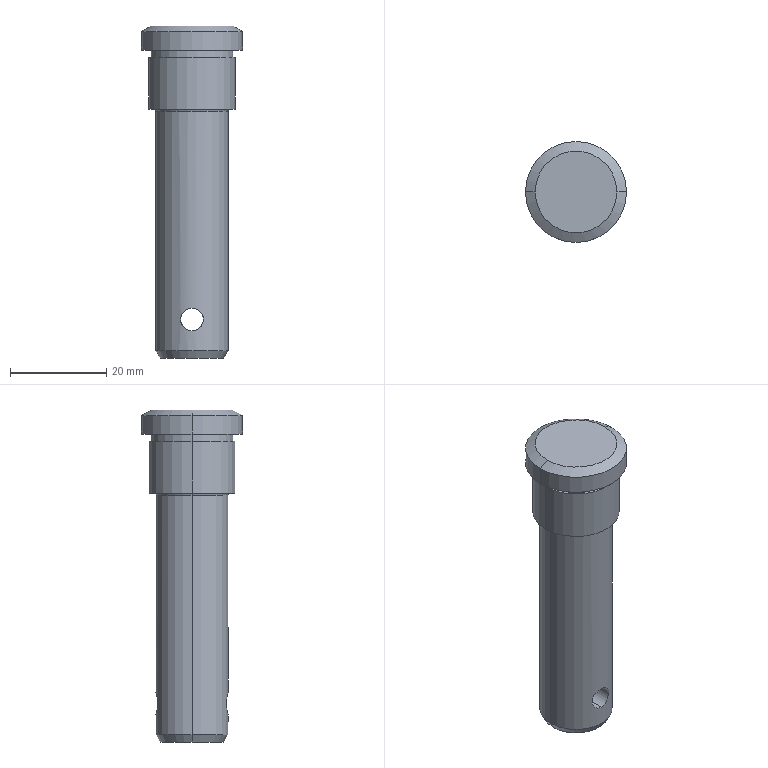Part | STEP file | PERNO POLEA_PERNO V2 | 1 solid | 21 faces | box 21 x 21 x 69 mm | volume 13594 mm3 | cylinder 10 | plane 5 | cone 4 | torus 2 | commonest cylinder face diameters 4.76 x2 15 x2 17 x2 18 x2 21 x2
STEP:
#1=CARTESIAN_POINT('',(7.5,0.,-17.7));
#2=VERTEX_POINT('',#1);
#3=CARTESIAN_POINT('',(-7.5,0.,-17.7));
#4=VERTEX_POINT('',#3);
#5=CARTESIAN_POINT('',(0.,0.,-17.7));
#6=DIRECTION('',(0.,0.,-1.));
#7=DIRECTION('',(-1.,0.,0.));
#8=AXIS2_PLACEMENT_3D('',#5,#6,#7);
#9=CIRCLE('',#8,7.5);
#10=EDGE_CURVE('',#2,#4,#9,.T.);
#11=ORIENTED_EDGE('',*,*,#10,.F.);
#12=CARTESIAN_POINT('',(7.9,0.,-17.3));
#13=VERTEX_POINT('',#12);
#14=CARTESIAN_POINT('',(7.9,0.,-17.7));
#15=DIRECTION('',(0.,1.,0.));
#16=DIRECTION('',(-1.,0.,0.));
#17=AXIS2_PLACEMENT_3D('',#14,#15,#16);
#18=CIRCLE('',#17,0.4);
#19=EDGE_CURVE('',#2,#13,#18,.T.);
#20=ORIENTED_EDGE('',*,*,#19,.T.);
#21=CARTESIAN_POINT('',(-7.9,0.,-17.3));
#22=VERTEX_POINT('',#21);
#23=CARTESIAN_POINT('',(0.,0.,-17.3));
#24=DIRECTION('',(0.,0.,1.));
#25=DIRECTION('',(-1.,0.,0.));
#26=AXIS2_PLACEMENT_3D('',#23,#24,#25);
#27=CIRCLE('',#26,7.9);
#28=EDGE_CURVE('',#22,#13,#27,.T.);
#29=ORIENTED_EDGE('',*,*,#28,.F.);
#30=CARTESIAN_POINT('',(-7.9,0.,-17.7));
#31=DIRECTION('',(0.,-1.,0.));
#32=DIRECTION('',(0.,0.,-1.));
#33=AXIS2_PLACEMENT_3D('',#30,#31,#32);
#34=CIRCLE('',#33,0.4);
#35=EDGE_CURVE('',#4,#22,#34,.T.);
#36=ORIENTED_EDGE('',*,*,#35,.F.);
#37=EDGE_LOOP('',(#11,#20,#29,#36));
#38=FACE_OUTER_BOUND('',#37,.T.);
#39=CARTESIAN_POINT('',(0.,0.,-17.7));
#40=DIRECTION('',(0.,0.,-1.));
#41=DIRECTION('',(-1.,0.,0.));
#42=AXIS2_PLACEMENT_3D('',#39,#40,#41);
#43=TOROIDAL_SURFACE('',#42,7.9,0.4);
#44=ADVANCED_FACE('',(#38),#43,.F.);
#45=CARTESIAN_POINT('',(0.,-7.5,-63.38));
#46=VERTEX_POINT('',#45);
#47=CARTESIAN_POINT('',(0.,-7.5,-58.62));
#48=VERTEX_POINT('',#47);
#49=CARTESIAN_POINT('',(0.,-7.5,-63.38));
#50=CARTESIAN_POINT('',(-0.3119,-7.5,-63.38));
#51=CARTESIAN_POINT('',(-0.6269,-7.479,-63.317));
#52=CARTESIAN_POINT('',(-1.057,-7.426,-63.138));
#53=CARTESIAN_POINT('',(-1.197,-7.405,-63.063));
#54=CARTESIAN_POINT('',(-1.454,-7.359,-62.891));
#55=CARTESIAN_POINT('',(-1.573,-7.334,-62.793));
#56=CARTESIAN_POINT('',(-1.903,-7.258,-62.463));
#57=CARTESIAN_POINT('',(-2.077,-7.208,-62.204));
#58=CARTESIAN_POINT('',(-2.258,-7.152,-61.769));
#59=CARTESIAN_POINT('',(-2.303,-7.138,-61.621));
#60=CARTESIAN_POINT('',(-2.364,-7.118,-61.315));
#61=CARTESIAN_POINT('',(-2.38,-7.112,-61.157));
#62=CARTESIAN_POINT('',(-2.38,-7.112,-60.843));
#63=CARTESIAN_POINT('',(-2.365,-7.118,-60.688));
#64=CARTESIAN_POINT('',(-2.303,-7.138,-60.381));
#65=CARTESIAN_POINT('',(-2.257,-7.153,-60.229));
#66=CARTESIAN_POINT('',(-2.078,-7.207,-59.799));
#67=CARTESIAN_POINT('',(-1.901,-7.258,-59.536));
#68=CARTESIAN_POINT('',(-1.574,-7.334,-59.208));
#69=CARTESIAN_POINT('',(-1.453,-7.359,-59.109));
#70=CARTESIAN_POINT('',(-1.195,-7.405,-58.936));
#71=CARTESIAN_POINT('',(-1.059,-7.426,-58.863));
#72=CARTESIAN_POINT('',(-0.7718,-7.462,-58.743));
#73=CARTESIAN_POINT('',(-0.6199,-7.476,-58.697));
#74=CARTESIAN_POINT('',(-0.314,-7.495,-58.636));
#75=CARTESIAN_POINT('',(-0.1583,-7.5,-58.62));
#76=CARTESIAN_POINT('',(0.,-7.5,-58.62));
#77=B_SPLINE_CURVE_WITH_KNOTS('',3,(#49,#50,#51,#52,#53,#54,#55,#56,#57,#58,#59,#60,#61,#62,#63,#64,#65,#66,#67,#68,#69,#70,#71,#72,#73,#74,#75,#76),.UNSPECIFIED.,.F.,.F.,(4,2,2,2,2,2,2,2,2,2,2,2,2,4),(0.00749,0.008426,0.008894,0.009362,0.0103,0.01077,0.01123,0.0117,0.01217,0.01311,0.01357,0.01404,0.01451,0.01498),.UNSPECIFIED.);
#78=EDGE_CURVE('',#46,#48,#77,.T.);
#79=ORIENTED_EDGE('',*,*,#78,.F.);
#80=CARTESIAN_POINT('',(0.,7.5,-63.38));
#81=VERTEX_POINT('',#80);
#82=CARTESIAN_POINT('',(0.,-10.5,-63.38));
#83=DIRECTION('',(0.,1.,0.));
#84=VECTOR('',#83,1000.);
#85=LINE('',#82,#84);
#86=EDGE_CURVE('',#46,#81,#85,.T.);
#87=ORIENTED_EDGE('',*,*,#86,.T.);
#88=CARTESIAN_POINT('',(0.,7.5,-58.62));
#89=VERTEX_POINT('',#88);
#90=CARTESIAN_POINT('',(0.,7.5,-58.62));
#91=CARTESIAN_POINT('',(-0.1584,7.5,-58.62));
#92=CARTESIAN_POINT('',(-0.3139,7.495,-58.636));
#93=CARTESIAN_POINT('',(-0.6195,7.476,-58.697));
#94=CARTESIAN_POINT('',(-0.7712,7.462,-58.743));
#95=CARTESIAN_POINT('',(-1.059,7.426,-58.863));
#96=CARTESIAN_POINT('',(-1.195,7.405,-58.936));
#97=CARTESIAN_POINT('',(-1.453,7.359,-59.109));
#98=CARTESIAN_POINT('',(-1.575,7.334,-59.209));
#99=CARTESIAN_POINT('',(-1.902,7.258,-59.536));
#100=CARTESIAN_POINT('',(-2.078,7.207,-59.8));
#101=CARTESIAN_POINT('',(-2.257,7.153,-60.229));
#102=CARTESIAN_POINT('',(-2.303,7.138,-60.38));
#103=CARTESIAN_POINT('',(-2.365,7.118,-60.687));
#104=CARTESIAN_POINT('',(-2.38,7.112,-60.842));
#105=CARTESIAN_POINT('',(-2.38,7.112,-61.155));
#106=CARTESIAN_POINT('',(-2.364,7.118,-61.314));
#107=CARTESIAN_POINT('',(-2.303,7.138,-61.62));
#108=CARTESIAN_POINT('',(-2.258,7.152,-61.769));
#109=CARTESIAN_POINT('',(-2.137,7.189,-62.059));
#110=CARTESIAN_POINT('',(-2.063,7.211,-62.196));
#111=CARTESIAN_POINT('',(-1.891,7.258,-62.453));
#112=CARTESIAN_POINT('',(-1.792,7.284,-62.574));
#113=CARTESIAN_POINT('',(-1.573,7.334,-62.793));
#114=CARTESIAN_POINT('',(-1.453,7.359,-62.891));
#115=CARTESIAN_POINT('',(-1.196,7.405,-63.063));
#116=CARTESIAN_POINT('',(-1.057,7.427,-63.138));
#117=CARTESIAN_POINT('',(-0.7702,7.462,-63.257));
#118=CARTESIAN_POINT('',(-0.6217,7.476,-63.303));
#119=CARTESIAN_POINT('',(-0.3139,7.495,-63.364));
#120=CARTESIAN_POINT('',(-0.156,7.5,-63.38));
#121=CARTESIAN_POINT('',(0.,7.5,-63.38));
#122=B_SPLINE_CURVE_WITH_KNOTS('',3,(#90,#91,#92,#93,#94,#95,#96,#97,#98,#99,#100,#101,#102,#103,#104,#105,#106,#107,#108,#109,#110,#111,#112,#113,#114,#115,#116,#117,#118,#119,#120,#121),.UNSPECIFIED.,.F.,.F.,(4,2,2,2,2,2,2,2,2,2,2,2,2,2,2,4),(0.,0.0004681,0.0009362,0.001404,0.001872,0.002809,0.003277,0.003745,0.004213,0.004681,0.005149,0.005617,0.006085,0.006553,0.007022,0.00749),.UNSPECIFIED.);
#123=EDGE_CURVE('',#89,#81,#122,.T.);
#124=ORIENTED_EDGE('',*,*,#123,.F.);
#125=CARTESIAN_POINT('',(0.,-10.5,-58.62));
#126=DIRECTION('',(0.,1.,0.));
#127=VECTOR('',#126,1000.);
#128=LINE('',#125,#127);
#129=EDGE_CURVE('',#48,#89,#128,.T.);
#130=ORIENTED_EDGE('',*,*,#129,.F.);
#131=EDGE_LOOP('',(#79,#87,#124,#130));
#132=FACE_OUTER_BOUND('',#131,.T.);
#133=CARTESIAN_POINT('',(0.,-10.5,-61.));
#134=DIRECTION('',(0.,1.,0.));
#135=DIRECTION('',(0.,0.,1.));
#136=AXIS2_PLACEMENT_3D('',#133,#134,#135);
#137=CYLINDRICAL_SURFACE('',#136,2.38);
#138=ADVANCED_FACE('',(#132),#137,.F.);
#139=CARTESIAN_POINT('',(-6.634,0.,-69.));
#140=VERTEX_POINT('',#139);
#141=CARTESIAN_POINT('',(6.634,0.,-69.));
#142=VERTEX_POINT('',#141);
#143=CARTESIAN_POINT('',(0.,0.,-69.));
#144=DIRECTION('',(0.,0.,-1.));
#145=DIRECTION('',(1.,0.,0.));
#146=AXIS2_PLACEMENT_3D('',#143,#144,#145);
#147=CIRCLE('',#146,6.634);
#148=EDGE_CURVE('',#140,#142,#147,.T.);
#149=ORIENTED_EDGE('',*,*,#148,.F.);
#150=CARTESIAN_POINT('',(-7.5,0.,-67.5));
#151=VERTEX_POINT('',#150);
#152=CARTESIAN_POINT('',(-7.5,0.,-67.5));
#153=DIRECTION('',(-0.5,0.,0.866));
#154=VECTOR('',#153,1000.);
#155=LINE('',#152,#154);
#156=EDGE_CURVE('',#140,#151,#155,.T.);
#157=ORIENTED_EDGE('',*,*,#156,.T.);
#158=CARTESIAN_POINT('',(7.5,0.,-67.5));
#159=VERTEX_POINT('',#158);
#160=CARTESIAN_POINT('',(0.,0.,-67.5));
#161=DIRECTION('',(0.,0.,1.));
#162=DIRECTION('',(1.,0.,0.));
#163=AXIS2_PLACEMENT_3D('',#160,#161,#162);
#164=CIRCLE('',#163,7.5);
#165=EDGE_CURVE('',#159,#151,#164,.T.);
#166=ORIENTED_EDGE('',*,*,#165,.F.);
#167=CARTESIAN_POINT('',(7.5,0.,-67.5));
#168=DIRECTION('',(0.5,0.,0.866));
#169=VECTOR('',#168,1000.);
#170=LINE('',#167,#169);
#171=EDGE_CURVE('',#142,#159,#170,.T.);
#172=ORIENTED_EDGE('',*,*,#171,.F.);
#173=EDGE_LOOP('',(#149,#157,#166,#172));
#174=FACE_OUTER_BOUND('',#173,.T.);
#175=CARTESIAN_POINT('',(0.,0.,-67.5));
#176=DIRECTION('',(0.,0.,1.));
#177=DIRECTION('',(1.,0.,0.));
#178=AXIS2_PLACEMENT_3D('',#175,#176,#177);
#179=CONICAL_SURFACE('',#178,7.5,0.5236);
#180=ADVANCED_FACE('',(#174),#179,.T.);
#181=CARTESIAN_POINT('',(8.5,0.,0.));
#182=VERTEX_POINT('',#181);
#183=CARTESIAN_POINT('',(-8.5,0.,0.));
#184=VERTEX_POINT('',#183);
#185=CARTESIAN_POINT('',(0.,0.,0.));
#186=DIRECTION('',(0.,0.,1.));
#187=DIRECTION('',(-1.,0.,0.));
#188=AXIS2_PLACEMENT_3D('',#185,#186,#187);
#189=CIRCLE('',#188,8.5);
#190=EDGE_CURVE('',#182,#184,#189,.T.);
#191=ORIENTED_EDGE('',*,*,#190,.F.);
#192=CARTESIAN_POINT('',(10.5,0.,-1.155));
#193=VERTEX_POINT('',#192);
#194=CARTESIAN_POINT('',(8.5,0.,0.));
#195=DIRECTION('',(0.866,0.,-0.5));
#196=VECTOR('',#195,1000.);
#197=LINE('',#194,#196);
#198=EDGE_CURVE('',#182,#193,#197,.T.);
#199=ORIENTED_EDGE('',*,*,#198,.T.);
#200=CARTESIAN_POINT('',(-10.5,0.,-1.155));
#201=VERTEX_POINT('',#200);
#202=CARTESIAN_POINT('',(0.,0.,-1.155));
#203=DIRECTION('',(0.,0.,-1.));
#204=DIRECTION('',(-1.,0.,0.));
#205=AXIS2_PLACEMENT_3D('',#202,#203,#204);
#206=CIRCLE('',#205,10.5);
#207=EDGE_CURVE('',#201,#193,#206,.T.);
#208=ORIENTED_EDGE('',*,*,#207,.F.);
#209=CARTESIAN_POINT('',(-8.5,0.,0.));
#210=DIRECTION('',(-0.866,0.,-0.5));
#211=VECTOR('',#210,1000.);
#212=LINE('',#209,#211);
#213=EDGE_CURVE('',#184,#201,#212,.T.);
#214=ORIENTED_EDGE('',*,*,#213,.F.);
#215=EDGE_LOOP('',(#191,#199,#208,#214));
#216=FACE_OUTER_BOUND('',#215,.T.);
#217=CARTESIAN_POINT('',(0.,0.,0.));
#218=DIRECTION('',(0.,0.,-1.));
#219=DIRECTION('',(-1.,0.,0.));
#220=AXIS2_PLACEMENT_3D('',#217,#218,#219);
#221=CONICAL_SURFACE('',#220,8.5,1.047);
#222=ADVANCED_FACE('',(#216),#221,.T.);
#223=CARTESIAN_POINT('',(10.5,0.,-5.));
#224=VERTEX_POINT('',#223);
#225=CARTESIAN_POINT('',(-10.5,0.,-5.));
#226=VERTEX_POINT('',#225);
#227=CARTESIAN_POINT('',(0.,0.,-5.));
#228=DIRECTION('',(0.,0.,1.));
#229=DIRECTION('',(1.,0.,0.));
#230=AXIS2_PLACEMENT_3D('',#227,#228,#229);
#231=CIRCLE('',#230,10.5);
#232=EDGE_CURVE('',#224,#226,#231,.T.);
#233=ORIENTED_EDGE('',*,*,#232,.T.);
#234=CARTESIAN_POINT('',(-10.5,0.,0.));
#235=DIRECTION('',(0.,0.,1.));
#236=VECTOR('',#235,1000.);
#237=LINE('',#234,#236);
#238=EDGE_CURVE('',#226,#201,#237,.T.);
#239=ORIENTED_EDGE('',*,*,#238,.T.);
#240=ORIENTED_EDGE('',*,*,#207,.T.);
#241=CARTESIAN_POINT('',(10.5,0.,0.));
#242=DIRECTION('',(0.,0.,1.));
#243=VECTOR('',#242,1000.);
#244=LINE('',#241,#243);
#245=EDGE_CURVE('',#224,#193,#244,.T.);
#246=ORIENTED_EDGE('',*,*,#245,.F.);
#247=EDGE_LOOP('',(#233,#239,#240,#246));
#248=FACE_OUTER_BOUND('',#247,.T.);
#249=CARTESIAN_POINT('',(0.,0.,0.));
#250=DIRECTION('',(0.,0.,1.));
#251=DIRECTION('',(1.,0.,0.));
#252=AXIS2_PLACEMENT_3D('',#249,#250,#251);
#253=CYLINDRICAL_SURFACE('',#252,10.5);
#254=ADVANCED_FACE('',(#248),#253,.T.);
#255=CARTESIAN_POINT('',(8.5,0.,-6.5));
#256=VERTEX_POINT('',#255);
#257=CARTESIAN_POINT('',(-8.5,0.,-6.5));
#258=VERTEX_POINT('',#257);
#259=CARTESIAN_POINT('',(0.,0.,-6.5));
#260=DIRECTION('',(0.,0.,1.));
#261=DIRECTION('',(1.,0.,0.));
#262=AXIS2_PLACEMENT_3D('',#259,#260,#261);
#263=CIRCLE('',#262,8.5);
#264=EDGE_CURVE('',#256,#258,#263,.T.);
#265=ORIENTED_EDGE('',*,*,#264,.T.);
#266=CARTESIAN_POINT('',(-8.5,0.,-5.));
#267=VERTEX_POINT('',#266);
#268=CARTESIAN_POINT('',(-8.5,0.,0.));
#269=DIRECTION('',(0.,0.,1.));
#270=VECTOR('',#269,1000.);
#271=LINE('',#268,#270);
#272=EDGE_CURVE('',#258,#267,#271,.T.);
#273=ORIENTED_EDGE('',*,*,#272,.T.);
#274=CARTESIAN_POINT('',(8.5,0.,-5.));
#275=VERTEX_POINT('',#274);
#276=CARTESIAN_POINT('',(0.,0.,-5.));
#277=DIRECTION('',(0.,0.,1.));
#278=DIRECTION('',(1.,0.,0.));
#279=AXIS2_PLACEMENT_3D('',#276,#277,#278);
#280=CIRCLE('',#279,8.5);
#281=EDGE_CURVE('',#275,#267,#280,.T.);
#282=ORIENTED_EDGE('',*,*,#281,.F.);
#283=CARTESIAN_POINT('',(8.5,0.,0.));
#284=DIRECTION('',(0.,0.,1.));
#285=VECTOR('',#284,1000.);
#286=LINE('',#283,#285);
#287=EDGE_CURVE('',#256,#275,#286,.T.);
#288=ORIENTED_EDGE('',*,*,#287,.F.);
#289=EDGE_LOOP('',(#265,#273,#282,#288));
#290=FACE_OUTER_BOUND('',#289,.T.);
#291=CARTESIAN_POINT('',(0.,0.,0.));
#292=DIRECTION('',(0.,0.,1.));
#293=DIRECTION('',(1.,0.,0.));
#294=AXIS2_PLACEMENT_3D('',#291,#292,#293);
#295=CYLINDRICAL_SURFACE('',#294,8.5);
#296=ADVANCED_FACE('',(#290),#295,.T.);
#297=ORIENTED_EDGE('',*,*,#123,.T.);
#298=CARTESIAN_POINT('',(0.,7.5,-63.38));
#299=CARTESIAN_POINT('',(0.3119,7.5,-63.38));
#300=CARTESIAN_POINT('',(0.6269,7.479,-63.317));
#301=CARTESIAN_POINT('',(1.057,7.426,-63.138));
#302=CARTESIAN_POINT('',(1.197,7.405,-63.063));
#303=CARTESIAN_POINT('',(1.454,7.359,-62.891));
#304=CARTESIAN_POINT('',(1.573,7.334,-62.793));
#305=CARTESIAN_POINT('',(1.903,7.258,-62.463));
#306=CARTESIAN_POINT('',(2.077,7.208,-62.204));
#307=CARTESIAN_POINT('',(2.258,7.152,-61.769));
#308=CARTESIAN_POINT('',(2.303,7.138,-61.621));
#309=CARTESIAN_POINT('',(2.364,7.118,-61.315));
#310=CARTESIAN_POINT('',(2.38,7.112,-61.157));
#311=CARTESIAN_POINT('',(2.38,7.112,-60.843));
#312=CARTESIAN_POINT('',(2.365,7.118,-60.688));
#313=CARTESIAN_POINT('',(2.303,7.138,-60.381));
#314=CARTESIAN_POINT('',(2.257,7.153,-60.229));
#315=CARTESIAN_POINT('',(2.078,7.207,-59.799));
#316=CARTESIAN_POINT('',(1.901,7.258,-59.536));
#317=CARTESIAN_POINT('',(1.574,7.334,-59.208));
#318=CARTESIAN_POINT('',(1.453,7.359,-59.109));
#319=CARTESIAN_POINT('',(1.195,7.405,-58.936));
#320=CARTESIAN_POINT('',(1.059,7.426,-58.863));
#321=CARTESIAN_POINT('',(0.7718,7.462,-58.743));
#322=CARTESIAN_POINT('',(0.6199,7.476,-58.697));
#323=CARTESIAN_POINT('',(0.314,7.495,-58.636));
#324=CARTESIAN_POINT('',(0.1583,7.5,-58.62));
#325=CARTESIAN_POINT('',(0.,7.5,-58.62));
#326=B_SPLINE_CURVE_WITH_KNOTS('',3,(#298,#299,#300,#301,#302,#303,#304,#305,#306,#307,#308,#309,#310,#311,#312,#313,#314,#315,#316,#317,#318,#319,#320,#321,#322,#323,#324,#325),.UNSPECIFIED.,.F.,.F.,(4,2,2,2,2,2,2,2,2,2,2,2,2,4),(0.00749,0.008426,0.008894,0.009362,0.0103,0.01077,0.01123,0.0117,0.01217,0.01311,0.01357,0.01404,0.01451,0.01498),.UNSPECIFIED.);
#327=EDGE_CURVE('',#81,#89,#326,.T.);
#328=ORIENTED_EDGE('',*,*,#327,.T.);
#329=EDGE_LOOP('',(#297,#328));
#330=FACE_BOUND('',#329,.T.);
#331=ORIENTED_EDGE('',*,*,#165,.T.);
#332=CARTESIAN_POINT('',(-7.5,0.,0.));
#333=DIRECTION('',(0.,0.,1.));
#334=VECTOR('',#333,1000.);
#335=LINE('',#332,#334);
#336=EDGE_CURVE('',#151,#4,#335,.T.);
#337=ORIENTED_EDGE('',*,*,#336,.T.);
#338=CARTESIAN_POINT('',(0.,0.,-17.7));
#339=DIRECTION('',(0.,0.,-1.));
#340=DIRECTION('',(-1.,0.,0.));
#341=AXIS2_PLACEMENT_3D('',#338,#339,#340);
#342=CIRCLE('',#341,7.5);
#343=EDGE_CURVE('',#4,#2,#342,.T.);
#344=ORIENTED_EDGE('',*,*,#343,.T.);
#345=CARTESIAN_POINT('',(7.5,0.,0.));
#346=DIRECTION('',(0.,0.,1.));
#347=VECTOR('',#346,1000.);
#348=LINE('',#345,#347);
#349=EDGE_CURVE('',#159,#2,#348,.T.);
#350=ORIENTED_EDGE('',*,*,#349,.F.);
#351=EDGE_LOOP('',(#331,#337,#344,#350));
#352=FACE_OUTER_BOUND('',#351,.T.);
#353=CARTESIAN_POINT('',(0.,0.,0.));
#354=DIRECTION('',(0.,0.,1.));
#355=DIRECTION('',(1.,0.,0.));
#356=AXIS2_PLACEMENT_3D('',#353,#354,#355);
#357=CYLINDRICAL_SURFACE('',#356,7.5);
#358=ADVANCED_FACE('',(#330,#352),#357,.T.);
#359=CARTESIAN_POINT('',(-9.,0.,-17.3));
#360=VERTEX_POINT('',#359);
#361=CARTESIAN_POINT('',(9.,0.,-17.3));
#362=VERTEX_POINT('',#361);
#363=CARTESIAN_POINT('',(0.,0.,-17.3));
#364=DIRECTION('',(0.,0.,-1.));
#365=DIRECTION('',(-1.,0.,0.));
#366=AXIS2_PLACEMENT_3D('',#363,#364,#365);
#367=CIRCLE('',#366,9.);
#368=EDGE_CURVE('',#360,#362,#367,.T.);
#369=ORIENTED_EDGE('',*,*,#368,.F.);
#370=CARTESIAN_POINT('',(-9.,0.,-6.5));
#371=VERTEX_POINT('',#370);
#372=CARTESIAN_POINT('',(-9.,0.,-17.3));
#373=DIRECTION('',(0.,0.,1.));
#374=VECTOR('',#373,1000.);
#375=LINE('',#372,#374);
#376=EDGE_CURVE('',#360,#371,#375,.T.);
#377=ORIENTED_EDGE('',*,*,#376,.T.);
#378=CARTESIAN_POINT('',(9.,0.,-6.5));
#379=VERTEX_POINT('',#378);
#380=CARTESIAN_POINT('',(0.,0.,-6.5));
#381=DIRECTION('',(0.,0.,1.));
#382=DIRECTION('',(1.,0.,0.));
#383=AXIS2_PLACEMENT_3D('',#380,#381,#382);
#384=CIRCLE('',#383,9.);
#385=EDGE_CURVE('',#379,#371,#384,.T.);
#386=ORIENTED_EDGE('',*,*,#385,.F.);
#387=CARTESIAN_POINT('',(9.,0.,-17.3));
#388=DIRECTION('',(0.,0.,1.));
#389=VECTOR('',#388,1000.);
#390=LINE('',#387,#389);
#391=EDGE_CURVE('',#362,#379,#390,.T.);
#392=ORIENTED_EDGE('',*,*,#391,.F.);
#393=EDGE_LOOP('',(#369,#377,#386,#392));
#394=FACE_OUTER_BOUND('',#393,.T.);
#395=CARTESIAN_POINT('',(0.,0.,-17.3));
#396=DIRECTION('',(0.,0.,1.));
#397=DIRECTION('',(1.,0.,0.));
#398=AXIS2_PLACEMENT_3D('',#395,#396,#397);
#399=CYLINDRICAL_SURFACE('',#398,9.);
#400=ADVANCED_FACE('',(#394),#399,.T.);
#401=ORIENTED_EDGE('',*,*,#376,.F.);
#402=CARTESIAN_POINT('',(0.,0.,-17.3));
#403=DIRECTION('',(0.,0.,-1.));
#404=DIRECTION('',(-1.,0.,0.));
#405=AXIS2_PLACEMENT_3D('',#402,#403,#404);
#406=CIRCLE('',#405,9.);
#407=EDGE_CURVE('',#362,#360,#406,.T.);
#408=ORIENTED_EDGE('',*,*,#407,.F.);
#409=ORIENTED_EDGE('',*,*,#391,.T.);
#410=CARTESIAN_POINT('',(0.,0.,-6.5));
#411=DIRECTION('',(0.,0.,1.));
#412=DIRECTION('',(1.,0.,0.));
#413=AXIS2_PLACEMENT_3D('',#410,#411,#412);
#414=CIRCLE('',#413,9.);
#415=EDGE_CURVE('',#371,#379,#414,.T.);
#416=ORIENTED_EDGE('',*,*,#415,.F.);
#417=EDGE_LOOP('',(#401,#408,#409,#416));
#418=FACE_OUTER_BOUND('',#417,.T.);
#419=CARTESIAN_POINT('',(0.,0.,-17.3));
#420=DIRECTION('',(0.,0.,1.));
#421=DIRECTION('',(1.,0.,0.));
#422=AXIS2_PLACEMENT_3D('',#419,#420,#421);
#423=CYLINDRICAL_SURFACE('',#422,9.);
#424=ADVANCED_FACE('',(#418),#423,.T.);
#425=ORIENTED_EDGE('',*,*,#28,.T.);
#426=CARTESIAN_POINT('',(0.,0.,-17.3));
#427=DIRECTION('',(0.,0.,1.));
#428=DIRECTION('',(-1.,0.,0.));
#429=AXIS2_PLACEMENT_3D('',#426,#427,#428);
#430=CIRCLE('',#429,7.9);
#431=EDGE_CURVE('',#13,#22,#430,.T.);
#432=ORIENTED_EDGE('',*,*,#431,.T.);
#433=EDGE_LOOP('',(#425,#432));
#434=FACE_BOUND('',#433,.T.);
#435=ORIENTED_EDGE('',*,*,#407,.T.);
#436=ORIENTED_EDGE('',*,*,#368,.T.);
#437=EDGE_LOOP('',(#435,#436));
#438=FACE_OUTER_BOUND('',#437,.T.);
#439=CARTESIAN_POINT('',(0.,0.,-17.3));
#440=DIRECTION('',(0.,0.,-1.));
#441=DIRECTION('',(-1.,0.,0.));
#442=AXIS2_PLACEMENT_3D('',#439,#440,#441);
#443=PLANE('',#442);
#444=ADVANCED_FACE('',(#434,#438),#443,.T.);
#445=CARTESIAN_POINT('',(0.,0.,-69.));
#446=DIRECTION('',(0.,0.,-1.));
#447=DIRECTION('',(1.,0.,0.));
#448=AXIS2_PLACEMENT_3D('',#445,#446,#447);
#449=CIRCLE('',#448,6.634);
#450=EDGE_CURVE('',#142,#140,#449,.T.);
#451=ORIENTED_EDGE('',*,*,#450,.T.);
#452=ORIENTED_EDGE('',*,*,#148,.T.);
#453=EDGE_LOOP('',(#451,#452));
#454=FACE_OUTER_BOUND('',#453,.T.);
#455=CARTESIAN_POINT('',(0.,7.5,-69.));
#456=DIRECTION('',(0.,0.,1.));
#457=DIRECTION('',(1.,0.,0.));
#458=AXIS2_PLACEMENT_3D('',#455,#456,#457);
#459=PLANE('',#458);
#460=ADVANCED_FACE('',(#454),#459,.F.);
#461=ORIENTED_EDGE('',*,*,#336,.F.);
#462=CARTESIAN_POINT('',(0.,0.,-67.5));
#463=DIRECTION('',(0.,0.,1.));
#464=DIRECTION('',(1.,0.,0.));
#465=AXIS2_PLACEMENT_3D('',#462,#463,#464);
#466=CIRCLE('',#465,7.5);
#467=EDGE_CURVE('',#151,#159,#466,.T.);
#468=ORIENTED_EDGE('',*,*,#467,.T.);
#469=ORIENTED_EDGE('',*,*,#349,.T.);
#470=ORIENTED_EDGE('',*,*,#10,.T.);
#471=EDGE_LOOP('',(#461,#468,#469,#470));
#472=FACE_OUTER_BOUND('',#471,.T.);
#473=CARTESIAN_POINT('',(0.,-7.5,-58.62));
#474=CARTESIAN_POINT('',(0.1584,-7.5,-58.62));
#475=CARTESIAN_POINT('',(0.3139,-7.495,-58.636));
#476=CARTESIAN_POINT('',(0.6195,-7.476,-58.697));
#477=CARTESIAN_POINT('',(0.7712,-7.462,-58.743));
#478=CARTESIAN_POINT('',(1.059,-7.426,-58.863));
#479=CARTESIAN_POINT('',(1.195,-7.405,-58.936));
#480=CARTESIAN_POINT('',(1.453,-7.359,-59.109));
#481=CARTESIAN_POINT('',(1.575,-7.334,-59.209));
#482=CARTESIAN_POINT('',(1.902,-7.258,-59.536));
#483=CARTESIAN_POINT('',(2.078,-7.207,-59.8));
#484=CARTESIAN_POINT('',(2.257,-7.153,-60.229));
#485=CARTESIAN_POINT('',(2.303,-7.138,-60.38));
#486=CARTESIAN_POINT('',(2.365,-7.118,-60.687));
#487=CARTESIAN_POINT('',(2.38,-7.112,-60.842));
#488=CARTESIAN_POINT('',(2.38,-7.112,-61.155));
#489=CARTESIAN_POINT('',(2.364,-7.118,-61.314));
#490=CARTESIAN_POINT('',(2.303,-7.138,-61.62));
#491=CARTESIAN_POINT('',(2.258,-7.152,-61.769));
#492=CARTESIAN_POINT('',(2.137,-7.189,-62.059));
#493=CARTESIAN_POINT('',(2.063,-7.211,-62.196));
#494=CARTESIAN_POINT('',(1.891,-7.258,-62.453));
#495=CARTESIAN_POINT('',(1.792,-7.284,-62.574));
#496=CARTESIAN_POINT('',(1.573,-7.334,-62.793));
#497=CARTESIAN_POINT('',(1.453,-7.359,-62.891));
#498=CARTESIAN_POINT('',(1.196,-7.405,-63.063));
#499=CARTESIAN_POINT('',(1.057,-7.427,-63.138));
#500=CARTESIAN_POINT('',(0.7702,-7.462,-63.257));
#501=CARTESIAN_POINT('',(0.6217,-7.476,-63.303));
#502=CARTESIAN_POINT('',(0.3139,-7.495,-63.364));
#503=CARTESIAN_POINT('',(0.156,-7.5,-63.38));
#504=CARTESIAN_POINT('',(0.,-7.5,-63.38));
#505=B_SPLINE_CURVE_WITH_KNOTS('',3,(#473,#474,#475,#476,#477,#478,#479,#480,#481,#482,#483,#484,#485,#486,#487,#488,#489,#490,#491,#492,#493,#494,#495,#496,#497,#498,#499,#500,#501,#502,#503,#504),.UNSPECIFIED.,.F.,.F.,(4,2,2,2,2,2,2,2,2,2,2,2,2,2,2,4),(0.,0.0004681,0.0009362,0.001404,0.001872,0.002809,0.003277,0.003745,0.004213,0.004681,0.005149,0.005617,0.006085,0.006553,0.007022,0.00749),.UNSPECIFIED.);
#506=EDGE_CURVE('',#48,#46,#505,.T.);
#507=ORIENTED_EDGE('',*,*,#506,.T.);
#508=ORIENTED_EDGE('',*,*,#78,.T.);
#509=EDGE_LOOP('',(#507,#508));
#510=FACE_BOUND('',#509,.T.);
#511=CARTESIAN_POINT('',(0.,0.,0.));
#512=DIRECTION('',(0.,0.,1.));
#513=DIRECTION('',(1.,0.,0.));
#514=AXIS2_PLACEMENT_3D('',#511,#512,#513);
#515=CYLINDRICAL_SURFACE('',#514,7.5);
#516=ADVANCED_FACE('',(#472,#510),#515,.T.);
#517=ORIENTED_EDGE('',*,*,#264,.F.);
#518=CARTESIAN_POINT('',(0.,0.,-6.5));
#519=DIRECTION('',(0.,0.,1.));
#520=DIRECTION('',(1.,0.,0.));
#521=AXIS2_PLACEMENT_3D('',#518,#519,#520);
#522=CIRCLE('',#521,8.5);
#523=EDGE_CURVE('',#258,#256,#522,.T.);
#524=ORIENTED_EDGE('',*,*,#523,.F.);
#525=EDGE_LOOP('',(#517,#524));
#526=FACE_BOUND('',#525,.T.);
#527=ORIENTED_EDGE('',*,*,#385,.T.);
#528=ORIENTED_EDGE('',*,*,#415,.T.);
#529=EDGE_LOOP('',(#527,#528));
#530=FACE_OUTER_BOUND('',#529,.T.);
#531=CARTESIAN_POINT('',(-23.264,0.,-6.5));
#532=DIRECTION('',(0.,0.,1.));
#533=DIRECTION('',(1.,0.,0.));
#534=AXIS2_PLACEMENT_3D('',#531,#532,#533);
#535=PLANE('',#534);
#536=ADVANCED_FACE('',(#526,#530),#535,.T.);
#537=ORIENTED_EDGE('',*,*,#272,.F.);
#538=ORIENTED_EDGE('',*,*,#523,.T.);
#539=ORIENTED_EDGE('',*,*,#287,.T.);
#540=CARTESIAN_POINT('',(0.,0.,-5.));
#541=DIRECTION('',(0.,0.,1.));
#542=DIRECTION('',(1.,0.,0.));
#543=AXIS2_PLACEMENT_3D('',#540,#541,#542);
#544=CIRCLE('',#543,8.5);
#545=EDGE_CURVE('',#267,#275,#544,.T.);
#546=ORIENTED_EDGE('',*,*,#545,.F.);
#547=EDGE_LOOP('',(#537,#538,#539,#546));
#548=FACE_OUTER_BOUND('',#547,.T.);
#549=CARTESIAN_POINT('',(0.,0.,0.));
#550=DIRECTION('',(0.,0.,1.));
#551=DIRECTION('',(1.,0.,0.));
#552=AXIS2_PLACEMENT_3D('',#549,#550,#551);
#553=CYLINDRICAL_SURFACE('',#552,8.5);
#554=ADVANCED_FACE('',(#548),#553,.T.);
#555=CARTESIAN_POINT('',(0.,0.,0.));
#556=DIRECTION('',(0.,0.,1.));
#557=DIRECTION('',(-1.,0.,0.));
#558=AXIS2_PLACEMENT_3D('',#555,#556,#557);
#559=CIRCLE('',#558,8.5);
#560=EDGE_CURVE('',#184,#182,#559,.T.);
#561=ORIENTED_EDGE('',*,*,#560,.T.);
#562=ORIENTED_EDGE('',*,*,#190,.T.);
#563=EDGE_LOOP('',(#561,#562));
#564=FACE_OUTER_BOUND('',#563,.T.);
#565=CARTESIAN_POINT('',(0.,0.,0.));
#566=DIRECTION('',(0.,0.,-1.));
#567=DIRECTION('',(-1.,0.,0.));
#568=AXIS2_PLACEMENT_3D('',#565,#566,#567);
#569=PLANE('',#568);
#570=ADVANCED_FACE('',(#564),#569,.F.);
#571=ORIENTED_EDGE('',*,*,#238,.F.);
#572=CARTESIAN_POINT('',(0.,0.,-5.));
#573=DIRECTION('',(0.,0.,1.));
#574=DIRECTION('',(1.,0.,0.));
#575=AXIS2_PLACEMENT_3D('',#572,#573,#574);
#576=CIRCLE('',#575,10.5);
#577=EDGE_CURVE('',#226,#224,#576,.T.);
#578=ORIENTED_EDGE('',*,*,#577,.T.);
#579=ORIENTED_EDGE('',*,*,#245,.T.);
#580=CARTESIAN_POINT('',(0.,0.,-1.155));
#581=DIRECTION('',(0.,0.,-1.));
#582=DIRECTION('',(-1.,0.,0.));
#583=AXIS2_PLACEMENT_3D('',#580,#581,#582);
#584=CIRCLE('',#583,10.5);
#585=EDGE_CURVE('',#193,#201,#584,.T.);
#586=ORIENTED_EDGE('',*,*,#585,.T.);
#587=EDGE_LOOP('',(#571,#578,#579,#586));
#588=FACE_OUTER_BOUND('',#587,.T.);
#589=CARTESIAN_POINT('',(0.,0.,0.));
#590=DIRECTION('',(0.,0.,1.));
#591=DIRECTION('',(1.,0.,0.));
#592=AXIS2_PLACEMENT_3D('',#589,#590,#591);
#593=CYLINDRICAL_SURFACE('',#592,10.5);
#594=ADVANCED_FACE('',(#588),#593,.T.);
#595=ORIENTED_EDGE('',*,*,#232,.F.);
#596=ORIENTED_EDGE('',*,*,#577,.F.);
#597=EDGE_LOOP('',(#595,#596));
#598=FACE_OUTER_BOUND('',#597,.T.);
#599=ORIENTED_EDGE('',*,*,#281,.T.);
#600=ORIENTED_EDGE('',*,*,#545,.T.);
#601=EDGE_LOOP('',(#599,#600));
#602=FACE_BOUND('',#601,.T.);
#603=CARTESIAN_POINT('',(0.,10.5,-5.));
#604=DIRECTION('',(0.,0.,1.));
#605=DIRECTION('',(1.,0.,0.));
#606=AXIS2_PLACEMENT_3D('',#603,#604,#605);
#607=PLANE('',#606);
#608=ADVANCED_FACE('',(#598,#602),#607,.F.);
#609=ORIENTED_EDGE('',*,*,#198,.F.);
#610=ORIENTED_EDGE('',*,*,#560,.F.);
#611=ORIENTED_EDGE('',*,*,#213,.T.);
#612=ORIENTED_EDGE('',*,*,#585,.F.);
#613=EDGE_LOOP('',(#609,#610,#611,#612));
#614=FACE_OUTER_BOUND('',#613,.T.);
#615=CARTESIAN_POINT('',(0.,0.,0.));
#616=DIRECTION('',(0.,0.,-1.));
#617=DIRECTION('',(-1.,0.,0.));
#618=AXIS2_PLACEMENT_3D('',#615,#616,#617);
#619=CONICAL_SURFACE('',#618,8.5,1.047);
#620=ADVANCED_FACE('',(#614),#619,.T.);
#621=ORIENTED_EDGE('',*,*,#156,.F.);
#622=ORIENTED_EDGE('',*,*,#450,.F.);
#623=ORIENTED_EDGE('',*,*,#171,.T.);
#624=ORIENTED_EDGE('',*,*,#467,.F.);
#625=EDGE_LOOP('',(#621,#622,#623,#624));
#626=FACE_OUTER_BOUND('',#625,.T.);
#627=CARTESIAN_POINT('',(0.,0.,-67.5));
#628=DIRECTION('',(0.,0.,1.));
#629=DIRECTION('',(1.,0.,0.));
#630=AXIS2_PLACEMENT_3D('',#627,#628,#629);
#631=CONICAL_SURFACE('',#630,7.5,0.5236);
#632=ADVANCED_FACE('',(#626),#631,.T.);
#633=ORIENTED_EDGE('',*,*,#86,.F.);
#634=ORIENTED_EDGE('',*,*,#506,.F.);
#635=ORIENTED_EDGE('',*,*,#129,.T.);
#636=ORIENTED_EDGE('',*,*,#327,.F.);
#637=EDGE_LOOP('',(#633,#634,#635,#636));
#638=FACE_OUTER_BOUND('',#637,.T.);
#639=CARTESIAN_POINT('',(0.,-10.5,-61.));
#640=DIRECTION('',(0.,1.,0.));
#641=DIRECTION('',(0.,0.,1.));
#642=AXIS2_PLACEMENT_3D('',#639,#640,#641);
#643=CYLINDRICAL_SURFACE('',#642,2.38);
#644=ADVANCED_FACE('',(#638),#643,.F.);
#645=ORIENTED_EDGE('',*,*,#19,.F.);
#646=ORIENTED_EDGE('',*,*,#343,.F.);
#647=ORIENTED_EDGE('',*,*,#35,.T.);
#648=ORIENTED_EDGE('',*,*,#431,.F.);
#649=EDGE_LOOP('',(#645,#646,#647,#648));
#650=FACE_OUTER_BOUND('',#649,.T.);
#651=CARTESIAN_POINT('',(0.,0.,-17.7));
#652=DIRECTION('',(0.,0.,-1.));
#653=DIRECTION('',(-1.,0.,0.));
#654=AXIS2_PLACEMENT_3D('',#651,#652,#653);
#655=TOROIDAL_SURFACE('',#654,7.9,0.4);
#656=ADVANCED_FACE('',(#650),#655,.F.);
#657=CLOSED_SHELL('',(#44,#138,#180,#222,#254,#296,#358,#400,#424,#444,#460,#516,#536,#554,#570,#594,#608,#620,#632,#644,#656));
#658=MANIFOLD_SOLID_BREP('',#657);
#659=CARTESIAN_POINT('',(0.,0.,0.));
#660=DIRECTION('',(0.,0.,1.));
#661=DIRECTION('',(1.,0.,0.));
#662=AXIS2_PLACEMENT_3D('',#659,#660,#661);
#663=(LENGTH_UNIT()NAMED_UNIT(*)SI_UNIT(.MILLI.,.METRE.));
#664=UNCERTAINTY_MEASURE_WITH_UNIT(LENGTH_MEASURE(0.00001),#663,'','');
#665=(NAMED_UNIT(*)PLANE_ANGLE_UNIT()SI_UNIT($,.RADIAN.));
#666=(NAMED_UNIT(*)SI_UNIT($,.STERADIAN.)SOLID_ANGLE_UNIT());
#667=(GEOMETRIC_REPRESENTATION_CONTEXT(3)GLOBAL_UNCERTAINTY_ASSIGNED_CONTEXT((#664))GLOBAL_UNIT_ASSIGNED_CONTEXT((#663,#665,#666))REPRESENTATION_CONTEXT('',''));
#668=ADVANCED_BREP_SHAPE_REPRESENTATION('',(#658,#662),#667);